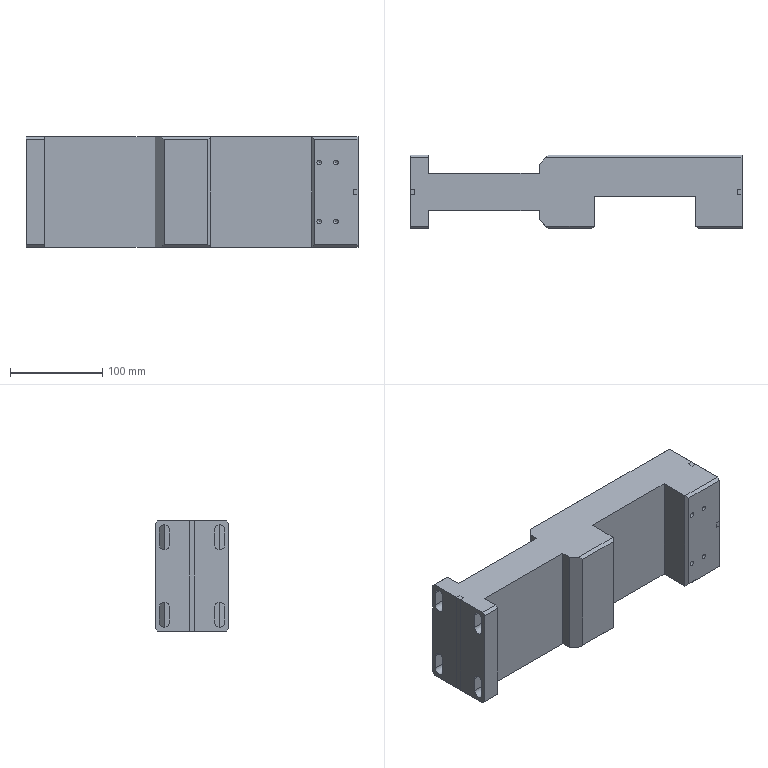Part | 2 solids | 160 faces | box 360 x 80 x 120 mm | volume 4738630 mm3 | plane 96 | cylinder 40 | cone 24 | commonest cylinder face diameters 5 x16 11 x16 6.8 x8